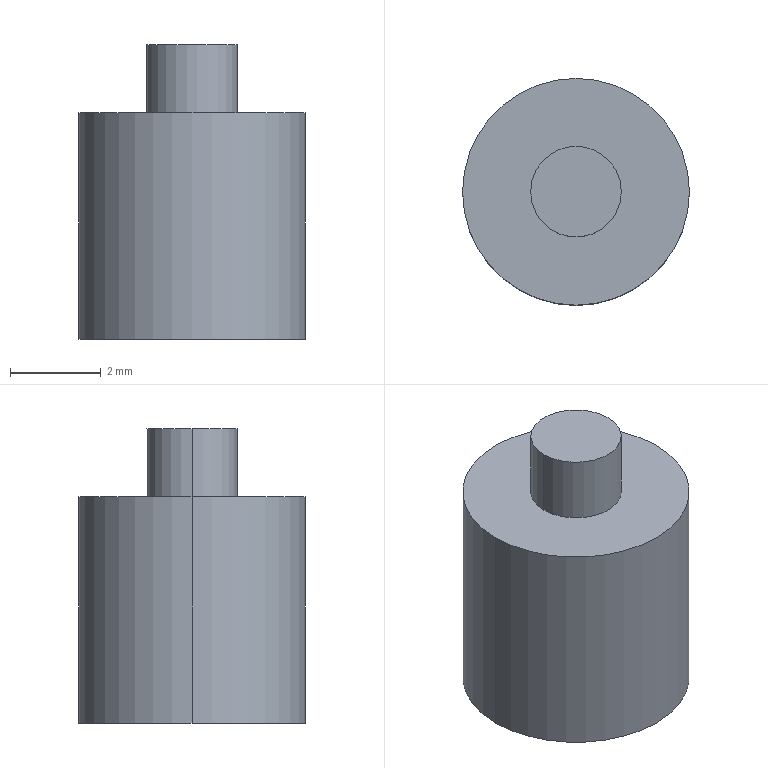Part | SolidWorks | features Extrusion 1, ICE 1, RevCut 1 | 1 solid | 9 faces | box 5 x 5 x 6.5 mm | volume 79.849 mm3 | cylinder 4 | plane 3 | sphere 2 | commonest cylinder face diameters 2 x2 5 x2
STEP:
#1=CARTESIAN_POINT('',(2.449,0.,0.));
#2=VERTEX_POINT('',#1);
#3=CARTESIAN_POINT('',(-2.449,0.,0.));
#4=VERTEX_POINT('',#3);
#5=CARTESIAN_POINT('',(0.,0.,0.));
#6=DIRECTION('',(0.,0.,1.));
#7=DIRECTION('',(1.,0.,0.));
#8=AXIS2_PLACEMENT_3D('',#5,#6,#7);
#9=CIRCLE('',#8,2.449);
#10=EDGE_CURVE('',#2,#4,#9,.T.);
#11=ORIENTED_EDGE('',*,*,#10,.F.);
#12=CARTESIAN_POINT('',(0.,0.,2.));
#13=VERTEX_POINT('',#12);
#14=CARTESIAN_POINT('',(0.,0.,-0.5));
#15=DIRECTION('',(0.,-1.,0.));
#16=DIRECTION('',(1.,0.,0.));
#17=AXIS2_PLACEMENT_3D('',#14,#15,#16);
#18=CIRCLE('',#17,2.5);
#19=EDGE_CURVE('',#2,#13,#18,.T.);
#20=ORIENTED_EDGE('',*,*,#19,.T.);
#21=CARTESIAN_POINT('',(0.,0.,-0.5));
#22=DIRECTION('',(0.,1.,0.));
#23=DIRECTION('',(0.,0.,1.));
#24=AXIS2_PLACEMENT_3D('',#21,#22,#23);
#25=CIRCLE('',#24,2.5);
#26=EDGE_CURVE('',#4,#13,#25,.T.);
#27=ORIENTED_EDGE('',*,*,#26,.F.);
#28=EDGE_LOOP('',(#11,#20,#27));
#29=FACE_OUTER_BOUND('',#28,.T.);
#30=CARTESIAN_POINT('',(0.,0.,-0.5));
#31=DIRECTION('',(0.,-1.,0.));
#32=DIRECTION('',(-1.,0.,0.));
#33=AXIS2_PLACEMENT_3D('',#30,#31,#32);
#34=SPHERICAL_SURFACE('',#33,2.5);
#35=ADVANCED_FACE('',(#29),#34,.F.);
#36=CARTESIAN_POINT('',(1.,0.,6.5));
#37=VERTEX_POINT('',#36);
#38=CARTESIAN_POINT('',(-1.,0.,6.5));
#39=VERTEX_POINT('',#38);
#40=CARTESIAN_POINT('',(0.,0.,6.5));
#41=DIRECTION('',(0.,0.,1.));
#42=DIRECTION('',(1.,0.,0.));
#43=AXIS2_PLACEMENT_3D('',#40,#41,#42);
#44=CIRCLE('',#43,1.);
#45=EDGE_CURVE('',#37,#39,#44,.T.);
#46=ORIENTED_EDGE('',*,*,#45,.F.);
#47=CARTESIAN_POINT('',(1.,0.,5.));
#48=VERTEX_POINT('',#47);
#49=CARTESIAN_POINT('',(1.,0.,6.5));
#50=DIRECTION('',(0.,0.,-1.));
#51=VECTOR('',#50,1000.);
#52=LINE('',#49,#51);
#53=EDGE_CURVE('',#37,#48,#52,.T.);
#54=ORIENTED_EDGE('',*,*,#53,.T.);
#55=CARTESIAN_POINT('',(-1.,0.,5.));
#56=VERTEX_POINT('',#55);
#57=CARTESIAN_POINT('',(0.,0.,5.));
#58=DIRECTION('',(0.,0.,1.));
#59=DIRECTION('',(1.,0.,0.));
#60=AXIS2_PLACEMENT_3D('',#57,#58,#59);
#61=CIRCLE('',#60,1.);
#62=EDGE_CURVE('',#48,#56,#61,.T.);
#63=ORIENTED_EDGE('',*,*,#62,.T.);
#64=CARTESIAN_POINT('',(-1.,0.,6.5));
#65=DIRECTION('',(0.,0.,-1.));
#66=VECTOR('',#65,1000.);
#67=LINE('',#64,#66);
#68=EDGE_CURVE('',#39,#56,#67,.T.);
#69=ORIENTED_EDGE('',*,*,#68,.F.);
#70=EDGE_LOOP('',(#46,#54,#63,#69));
#71=FACE_OUTER_BOUND('',#70,.T.);
#72=CARTESIAN_POINT('',(0.,0.,6.5));
#73=DIRECTION('',(0.,0.,-1.));
#74=DIRECTION('',(-1.,0.,0.));
#75=AXIS2_PLACEMENT_3D('',#72,#73,#74);
#76=CYLINDRICAL_SURFACE('',#75,1.);
#77=ADVANCED_FACE('',(#71),#76,.T.);
#78=CARTESIAN_POINT('',(2.5,0.,5.));
#79=VERTEX_POINT('',#78);
#80=CARTESIAN_POINT('',(-2.5,0.,5.));
#81=VERTEX_POINT('',#80);
#82=CARTESIAN_POINT('',(0.,0.,5.));
#83=DIRECTION('',(0.,0.,1.));
#84=DIRECTION('',(1.,0.,0.));
#85=AXIS2_PLACEMENT_3D('',#82,#83,#84);
#86=CIRCLE('',#85,2.5);
#87=EDGE_CURVE('',#79,#81,#86,.T.);
#88=ORIENTED_EDGE('',*,*,#87,.F.);
#89=CARTESIAN_POINT('',(2.5,0.,0.));
#90=VERTEX_POINT('',#89);
#91=CARTESIAN_POINT('',(2.5,0.,5.));
#92=DIRECTION('',(0.,0.,-1.));
#93=VECTOR('',#92,1000.);
#94=LINE('',#91,#93);
#95=EDGE_CURVE('',#79,#90,#94,.T.);
#96=ORIENTED_EDGE('',*,*,#95,.T.);
#97=CARTESIAN_POINT('',(-2.5,0.,0.));
#98=VERTEX_POINT('',#97);
#99=CARTESIAN_POINT('',(0.,0.,0.));
#100=DIRECTION('',(0.,0.,1.));
#101=DIRECTION('',(1.,0.,0.));
#102=AXIS2_PLACEMENT_3D('',#99,#100,#101);
#103=CIRCLE('',#102,2.5);
#104=EDGE_CURVE('',#90,#98,#103,.T.);
#105=ORIENTED_EDGE('',*,*,#104,.T.);
#106=CARTESIAN_POINT('',(-2.5,0.,5.));
#107=DIRECTION('',(0.,0.,-1.));
#108=VECTOR('',#107,1000.);
#109=LINE('',#106,#108);
#110=EDGE_CURVE('',#81,#98,#109,.T.);
#111=ORIENTED_EDGE('',*,*,#110,.F.);
#112=EDGE_LOOP('',(#88,#96,#105,#111));
#113=FACE_OUTER_BOUND('',#112,.T.);
#114=CARTESIAN_POINT('',(0.,0.,5.));
#115=DIRECTION('',(0.,0.,-1.));
#116=DIRECTION('',(-1.,0.,0.));
#117=AXIS2_PLACEMENT_3D('',#114,#115,#116);
#118=CYLINDRICAL_SURFACE('',#117,2.5);
#119=ADVANCED_FACE('',(#113),#118,.T.);
#120=ORIENTED_EDGE('',*,*,#95,.F.);
#121=CARTESIAN_POINT('',(0.,0.,5.));
#122=DIRECTION('',(0.,0.,1.));
#123=DIRECTION('',(1.,0.,0.));
#124=AXIS2_PLACEMENT_3D('',#121,#122,#123);
#125=CIRCLE('',#124,2.5);
#126=EDGE_CURVE('',#81,#79,#125,.T.);
#127=ORIENTED_EDGE('',*,*,#126,.F.);
#128=ORIENTED_EDGE('',*,*,#110,.T.);
#129=CARTESIAN_POINT('',(0.,0.,0.));
#130=DIRECTION('',(0.,0.,1.));
#131=DIRECTION('',(1.,0.,0.));
#132=AXIS2_PLACEMENT_3D('',#129,#130,#131);
#133=CIRCLE('',#132,2.5);
#134=EDGE_CURVE('',#98,#90,#133,.T.);
#135=ORIENTED_EDGE('',*,*,#134,.T.);
#136=EDGE_LOOP('',(#120,#127,#128,#135));
#137=FACE_OUTER_BOUND('',#136,.T.);
#138=CARTESIAN_POINT('',(0.,0.,5.));
#139=DIRECTION('',(0.,0.,-1.));
#140=DIRECTION('',(-1.,0.,0.));
#141=AXIS2_PLACEMENT_3D('',#138,#139,#140);
#142=CYLINDRICAL_SURFACE('',#141,2.5);
#143=ADVANCED_FACE('',(#137),#142,.T.);
#144=CARTESIAN_POINT('',(0.,0.,5.));
#145=DIRECTION('',(0.,0.,1.));
#146=DIRECTION('',(1.,0.,0.));
#147=AXIS2_PLACEMENT_3D('',#144,#145,#146);
#148=CIRCLE('',#147,1.);
#149=EDGE_CURVE('',#56,#48,#148,.T.);
#150=ORIENTED_EDGE('',*,*,#149,.F.);
#151=ORIENTED_EDGE('',*,*,#62,.F.);
#152=EDGE_LOOP('',(#150,#151));
#153=FACE_BOUND('',#152,.T.);
#154=ORIENTED_EDGE('',*,*,#126,.T.);
#155=ORIENTED_EDGE('',*,*,#87,.T.);
#156=EDGE_LOOP('',(#154,#155));
#157=FACE_OUTER_BOUND('',#156,.T.);
#158=CARTESIAN_POINT('',(0.,0.,5.));
#159=DIRECTION('',(0.,0.,1.));
#160=DIRECTION('',(1.,0.,0.));
#161=AXIS2_PLACEMENT_3D('',#158,#159,#160);
#162=PLANE('',#161);
#163=ADVANCED_FACE('',(#153,#157),#162,.T.);
#164=CARTESIAN_POINT('',(0.,0.,0.));
#165=DIRECTION('',(0.,0.,1.));
#166=DIRECTION('',(1.,0.,0.));
#167=AXIS2_PLACEMENT_3D('',#164,#165,#166);
#168=CIRCLE('',#167,2.449);
#169=EDGE_CURVE('',#4,#2,#168,.T.);
#170=ORIENTED_EDGE('',*,*,#169,.T.);
#171=ORIENTED_EDGE('',*,*,#10,.T.);
#172=EDGE_LOOP('',(#170,#171));
#173=FACE_BOUND('',#172,.T.);
#174=ORIENTED_EDGE('',*,*,#134,.F.);
#175=ORIENTED_EDGE('',*,*,#104,.F.);
#176=EDGE_LOOP('',(#174,#175));
#177=FACE_OUTER_BOUND('',#176,.T.);
#178=CARTESIAN_POINT('',(0.,0.,0.));
#179=DIRECTION('',(0.,0.,1.));
#180=DIRECTION('',(1.,0.,0.));
#181=AXIS2_PLACEMENT_3D('',#178,#179,#180);
#182=PLANE('',#181);
#183=ADVANCED_FACE('',(#173,#177),#182,.F.);
#184=ORIENTED_EDGE('',*,*,#53,.F.);
#185=CARTESIAN_POINT('',(0.,0.,6.5));
#186=DIRECTION('',(0.,0.,1.));
#187=DIRECTION('',(1.,0.,0.));
#188=AXIS2_PLACEMENT_3D('',#185,#186,#187);
#189=CIRCLE('',#188,1.);
#190=EDGE_CURVE('',#39,#37,#189,.T.);
#191=ORIENTED_EDGE('',*,*,#190,.F.);
#192=ORIENTED_EDGE('',*,*,#68,.T.);
#193=ORIENTED_EDGE('',*,*,#149,.T.);
#194=EDGE_LOOP('',(#184,#191,#192,#193));
#195=FACE_OUTER_BOUND('',#194,.T.);
#196=CARTESIAN_POINT('',(0.,0.,6.5));
#197=DIRECTION('',(0.,0.,-1.));
#198=DIRECTION('',(-1.,0.,0.));
#199=AXIS2_PLACEMENT_3D('',#196,#197,#198);
#200=CYLINDRICAL_SURFACE('',#199,1.);
#201=ADVANCED_FACE('',(#195),#200,.T.);
#202=ORIENTED_EDGE('',*,*,#190,.T.);
#203=ORIENTED_EDGE('',*,*,#45,.T.);
#204=EDGE_LOOP('',(#202,#203));
#205=FACE_OUTER_BOUND('',#204,.T.);
#206=CARTESIAN_POINT('',(0.,0.,6.5));
#207=DIRECTION('',(0.,0.,1.));
#208=DIRECTION('',(1.,0.,0.));
#209=AXIS2_PLACEMENT_3D('',#206,#207,#208);
#210=PLANE('',#209);
#211=ADVANCED_FACE('',(#205),#210,.T.);
#212=ORIENTED_EDGE('',*,*,#19,.F.);
#213=ORIENTED_EDGE('',*,*,#169,.F.);
#214=ORIENTED_EDGE('',*,*,#26,.T.);
#215=EDGE_LOOP('',(#212,#213,#214));
#216=FACE_OUTER_BOUND('',#215,.T.);
#217=CARTESIAN_POINT('',(0.,0.,-0.5));
#218=DIRECTION('',(0.,-1.,0.));
#219=DIRECTION('',(-1.,0.,0.));
#220=AXIS2_PLACEMENT_3D('',#217,#218,#219);
#221=SPHERICAL_SURFACE('',#220,2.5);
#222=ADVANCED_FACE('',(#216),#221,.F.);
#223=CLOSED_SHELL('',(#35,#77,#119,#143,#163,#183,#201,#211,#222));
#224=MANIFOLD_SOLID_BREP('',#223);
#225=CARTESIAN_POINT('',(0.,0.,0.));
#226=DIRECTION('',(0.,0.,1.));
#227=DIRECTION('',(1.,0.,0.));
#228=AXIS2_PLACEMENT_3D('',#225,#226,#227);
#229=(LENGTH_UNIT()NAMED_UNIT(*)SI_UNIT(.MILLI.,.METRE.));
#230=UNCERTAINTY_MEASURE_WITH_UNIT(LENGTH_MEASURE(0.00001),#229,'','');
#231=(NAMED_UNIT(*)PLANE_ANGLE_UNIT()SI_UNIT($,.RADIAN.));
#232=(NAMED_UNIT(*)SI_UNIT($,.STERADIAN.)SOLID_ANGLE_UNIT());
#233=(GEOMETRIC_REPRESENTATION_CONTEXT(3)GLOBAL_UNCERTAINTY_ASSIGNED_CONTEXT((#230))GLOBAL_UNIT_ASSIGNED_CONTEXT((#229,#231,#232))REPRESENTATION_CONTEXT('',''));
#234=ADVANCED_BREP_SHAPE_REPRESENTATION('',(#224,#228),#233);